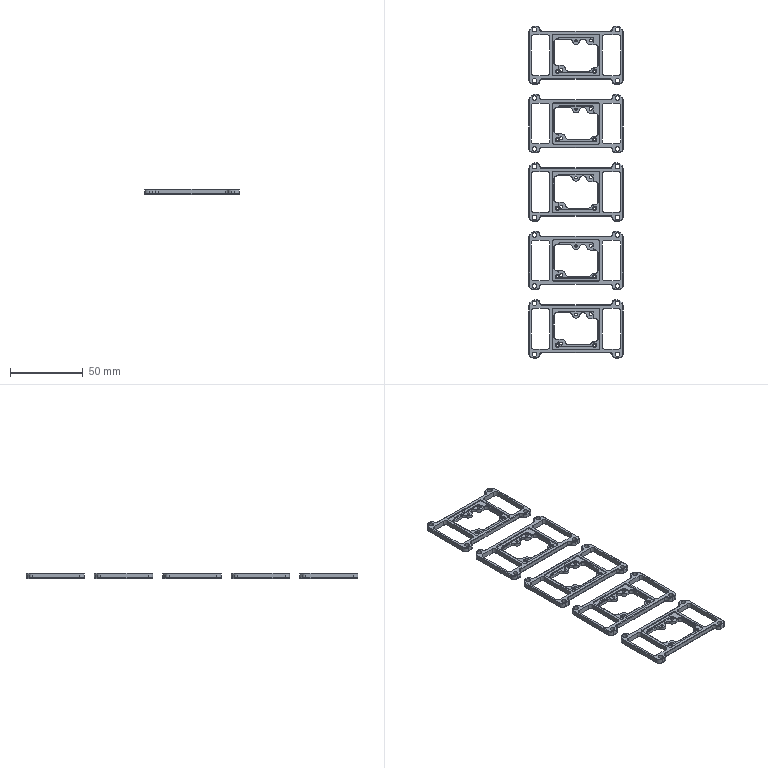NC program | NX | posted with a generic post | part box 65 x 228 x 3.5 mm
Lines 17082 to 18127 of 31259:
(ZLEVEL_PROFILE_COPY_COPY , TOOL : D1.5)
N34126 T17 M6
N34128 G54
N34130 G17 G0 G90 X-80.858 Y13.824 S9500 M3
N34132 G43 Z30. H17
N34134 Z0.4
N34136 G94 G1 Z-0.1 F1000.
N34138 X-80.633 Y13.954
N34140 X-80.552 Y13.994
N34142 X-80.558 Y14.084
N34144 Y15.05
N34146 G3 X-80.95 Y15.442 R0.392
N34148 G1 X-81.916
N34150 X-82.006 Y15.448
N34152 X-82.046 Y15.367
N34154 X-82.176 Y15.142
N34156 Z0.4
N34158 G0 X-80.915 Y13.767 Z0.3
N34160 G1 Z-0.2
N34162 X-80.69 Y13.897
N34164 X-80.61 Y13.936
N34166 X-80.615 Y14.026
N34168 Y15.05
N34170 G3 X-80.95 Y15.385 R0.335
N34172 G1 X-81.974
N34174 X-82.064 Y15.39
N34176 X-82.103 Y15.31
N34178 X-82.233 Y15.085
N34180 Z0.3
N34182 G0 X-80.973 Y13.709 Z0.2
N34184 G1 Z-0.3
N34186 X-80.748 Y13.839
N34188 X-80.667 Y13.879
N34190 X-80.673 Y13.969
N34192 Y15.05
N34194 G3 X-80.95 Y15.327 R0.277
N34196 G1 X-82.031
N34198 X-82.121 Y15.333
N34200 X-82.161 Y15.252
N34202 X-82.291 Y15.027
N34204 Z0.2
N34206 G0 X-81. Y13.682 Z0.1
N34208 G1 Z-0.4
N34210 X-80.775 Y13.812
N34212 X-80.694 Y13.852
N34214 X-80.7 Y13.942
N34216 Y15.05
N34218 G3 X-80.95 Y15.3 R0.25
N34220 G1 X-82.058
N34222 X-82.148 Y15.306
N34224 X-82.188 Y15.225
N34226 X-82.318 Y15.
N34228 Z0.1
N34230 G0 X-81. Y13.682 Z0.
N34232 G1 Z-0.5
N34234 X-80.775 Y13.812
N34236 X-80.694 Y13.852
N34238 X-80.7 Y13.942
N34240 Y15.05
N34242 G3 X-80.95 Y15.3 R0.25
N34244 G1 X-82.058
N34246 X-82.148 Y15.306
N34248 X-82.188 Y15.225
N34250 X-82.318 Y15.
N34252 Z0.
N34254 G0 X-81. Y13.682 Z-0.1
N34256 G1 Z-0.6
N34258 X-80.775 Y13.812
N34260 X-80.694 Y13.852
N34262 X-80.7 Y13.942
N34264 Y15.05
N34266 G3 X-80.95 Y15.3 R0.25
N34268 G1 X-82.058
N34270 X-82.148 Y15.306
N34272 X-82.188 Y15.225
N34274 X-82.318 Y15.
N34276 Z-0.1
N34278 G0 Z10.
N34280 X-105.824 Y15.142
N34282 Z0.4
N34284 G1 Z-0.1
N34286 X-105.954 Y15.367
N34288 X-105.994 Y15.448
N34290 X-106.084 Y15.442
N34292 X-107.05
N34294 G3 X-107.442 Y15.05 R0.392
N34296 G1 Y14.084
N34298 X-107.448 Y13.994
N34300 X-107.367 Y13.954
N34302 X-107.142 Y13.824
N34304 Z0.4
N34306 G0 X-105.767 Y15.085 Z0.3
N34308 G1 Z-0.2
N34310 X-105.897 Y15.31
N34312 X-105.936 Y15.39
N34314 X-106.026 Y15.385
N34316 X-107.05
N34318 G3 X-107.385 Y15.05 R0.335
N34320 G1 Y14.026
N34322 X-107.39 Y13.936
N34324 X-107.31 Y13.897
N34326 X-107.085 Y13.767
N34328 Z0.3
N34330 G0 X-105.709 Y15.027 Z0.2
N34332 G1 Z-0.3
N34334 X-105.839 Y15.252
N34336 X-105.879 Y15.333
N34338 X-105.969 Y15.327
N34340 X-107.05
N34342 G3 X-107.327 Y15.05 R0.277
N34344 G1 Y13.969
N34346 X-107.333 Y13.879
N34348 X-107.252 Y13.839
N34350 X-107.027 Y13.709
N34352 Z0.2
N34354 G0 X-105.682 Y15. Z0.1
N34356 G1 Z-0.4
N34358 X-105.812 Y15.225
N34360 X-105.852 Y15.306
N34362 X-105.942 Y15.3
N34364 X-107.05
N34366 G3 X-107.3 Y15.05 R0.25
N34368 G1 Y13.942
N34370 X-107.306 Y13.852
N34372 X-107.225 Y13.812
N34374 X-107. Y13.682
N34376 Z0.1
N34378 G0 X-105.682 Y15. Z0.
N34380 G1 Z-0.5
N34382 X-105.812 Y15.225
N34384 X-105.852 Y15.306
N34386 X-105.942 Y15.3
N34388 X-107.05
N34390 G3 X-107.3 Y15.05 R0.25
N34392 G1 Y13.942
N34394 X-107.306 Y13.852
N34396 X-107.225 Y13.812
N34398 X-107. Y13.682
N34400 Z0.
N34402 G0 X-105.682 Y15. Z-0.1
N34404 G1 Z-0.6
N34406 X-105.812 Y15.225
N34408 X-105.852 Y15.306
N34410 X-105.942 Y15.3
N34412 X-107.05
N34414 G3 X-107.3 Y15.05 R0.25
N34416 G1 Y13.942
N34418 X-107.306 Y13.852
N34420 X-107.225 Y13.812
N34422 X-107. Y13.682
N34424 Z-0.1
N34426 G0 Z10.
N34428 X-107.142 Y-13.824
N34430 Z0.4
N34432 G1 Z-0.1
N34434 X-107.367 Y-13.954
N34436 X-107.448 Y-13.994
N34438 X-107.442 Y-14.084
N34440 Y-15.05
N34442 G3 X-107.05 Y-15.442 R0.392
N34444 G1 X-106.084
N34446 X-105.994 Y-15.448
N34448 X-105.954 Y-15.367
N34450 X-105.824 Y-15.142
N34452 Z0.4
N34454 G0 X-107.085 Y-13.767 Z0.3
N34456 G1 Z-0.2
N34458 X-107.31 Y-13.897
N34460 X-107.39 Y-13.936
N34462 X-107.385 Y-14.026
N34464 Y-15.05
N34466 G3 X-107.05 Y-15.385 R0.335
N34468 G1 X-106.026
N34470 X-105.936 Y-15.39
N34472 X-105.897 Y-15.31
N34474 X-105.767 Y-15.085
N34476 Z0.3
N34478 G0 X-107.027 Y-13.709 Z0.2
N34480 G1 Z-0.3
N34482 X-107.252 Y-13.839
N34484 X-107.333 Y-13.879
N34486 X-107.327 Y-13.969
N34488 Y-15.05
N34490 G3 X-107.05 Y-15.327 R0.277
N34492 G1 X-105.969
N34494 X-105.879 Y-15.333
N34496 X-105.839 Y-15.252
N34498 X-105.709 Y-15.027
N34500 Z0.2
N34502 G0 X-107. Y-13.682 Z0.1
N34504 G1 Z-0.4
N34506 X-107.225 Y-13.812
N34508 X-107.306 Y-13.852
N34510 X-107.3 Y-13.942
N34512 Y-15.05
N34514 G3 X-107.05 Y-15.3 R0.25
N34516 G1 X-105.942
N34518 X-105.852 Y-15.306
N34520 X-105.812 Y-15.225
N34522 X-105.682 Y-15.
N34524 Z0.1
N34526 G0 X-107. Y-13.682 Z0.
N34528 G1 Z-0.5
N34530 X-107.225 Y-13.812
N34532 X-107.306 Y-13.852
N34534 X-107.3 Y-13.942
N34536 Y-15.05
N34538 G3 X-107.05 Y-15.3 R0.25
N34540 G1 X-105.942
N34542 X-105.852 Y-15.306
N34544 X-105.812 Y-15.225
N34546 X-105.682 Y-15.
N34548 Z0.
N34550 G0 X-107. Y-13.682 Z-0.1
N34552 G1 Z-0.6
N34554 X-107.225 Y-13.812
N34556 X-107.306 Y-13.852
N34558 X-107.3 Y-13.942
N34560 Y-15.05
N34562 G3 X-107.05 Y-15.3 R0.25
N34564 G1 X-105.942
N34566 X-105.852 Y-15.306
N34568 X-105.812 Y-15.225
N34570 X-105.682 Y-15.
N34572 Z-0.1
N34574 G0 Z10.
N34576 X-82.176 Y-15.142
N34578 Z0.4
N34580 G1 Z-0.1
N34582 X-82.046 Y-15.367
N34584 X-82.006 Y-15.448
N34586 X-81.916 Y-15.442
N34588 X-80.95
N34590 G3 X-80.558 Y-15.05 R0.392
N34592 G1 Y-14.084
N34594 X-80.552 Y-13.994
N34596 X-80.633 Y-13.954
N34598 X-80.858 Y-13.824
N34600 Z0.4
N34602 G0 X-82.233 Y-15.085 Z0.3
N34604 G1 Z-0.2
N34606 X-82.103 Y-15.31
N34608 X-82.064 Y-15.39
N34610 X-81.974 Y-15.385
N34612 X-80.95
N34614 G3 X-80.615 Y-15.05 R0.335
N34616 G1 Y-14.026
N34618 X-80.61 Y-13.936
N34620 X-80.69 Y-13.897
N34622 X-80.915 Y-13.767
N34624 Z0.3
N34626 G0 X-82.291 Y-15.027 Z0.2
N34628 G1 Z-0.3
N34630 X-82.161 Y-15.252
N34632 X-82.121 Y-15.333
N34634 X-82.031 Y-15.327
N34636 X-80.95
N34638 G3 X-80.673 Y-15.05 R0.277
N34640 G1 Y-13.969
N34642 X-80.667 Y-13.879
N34644 X-80.748 Y-13.839
N34646 X-80.973 Y-13.709
N34648 Z0.2
N34650 G0 X-82.318 Y-15. Z0.1
N34652 G1 Z-0.4
N34654 X-82.188 Y-15.225
N34656 X-82.148 Y-15.306
N34658 X-82.058 Y-15.3
N34660 X-80.95
N34662 G3 X-80.7 Y-15.05 R0.25
N34664 G1 Y-13.942
N34666 X-80.694 Y-13.852
N34668 X-80.775 Y-13.812
N34670 X-81. Y-13.682
N34672 Z0.1
N34674 G0 X-82.319 Y-15. Z0.
N34676 G1 Z-0.5
N34678 X-82.189 Y-15.225
N34680 X-82.149 Y-15.306
N34682 X-82.059 Y-15.3
N34684 X-80.95
N34686 G3 X-80.7 Y-15.05 R0.25
N34688 G1 Y-13.941
N34690 X-80.694 Y-13.851
N34692 X-80.775 Y-13.811
N34694 X-81. Y-13.681
N34696 Z0.
N34698 G0 X-82.319 Y-15. Z-0.1
N34700 G1 Z-0.6
N34702 X-82.189 Y-15.225
N34704 X-82.149 Y-15.306
N34706 X-82.059 Y-15.3
N34708 X-80.95
N34710 G3 X-80.7 Y-15.05 R0.25
N34712 G1 Y-13.941
N34714 X-80.694 Y-13.851
N34716 X-80.775 Y-13.811
N34718 X-81. Y-13.681
N34720 Z-0.1
N34722 G0 Z10.
N34724 X-76.182 Y28.948
N34726 Z0.4
N34728 G1 Z-0.1
N34730 X-76.37 Y29.275
N34732 X-76.41 Y29.356
N34734 X-76.5 Y29.35
N34736 G3 X-77.35 Y28.5 R0.85
N34738 X-76.5 Y29.35 R-0.85
N34740 G1 X-76.59 Y29.356
N34742 X-76.63 Y29.275
N34744 X-76.818 Y28.948
N34746 Z0.4
N34748 G0 X-76.182 Z0.3
N34750 G1 Z-0.2
N34752 X-76.37 Y29.275
N34754 X-76.41 Y29.356
N34756 X-76.5 Y29.35
N34758 G3 X-77.35 Y28.5 R0.85
N34760 X-76.5 Y29.35 R-0.85
N34762 G1 X-76.59 Y29.356
N34764 X-76.63 Y29.275
N34766 X-76.818 Y28.948
N34768 Z0.3
N34770 G0 X-76.182 Z0.2
N34772 G1 Z-0.3
N34774 X-76.37 Y29.275
N34776 X-76.41 Y29.356
N34778 X-76.5 Y29.35
N34780 G3 X-77.35 Y28.5 R0.85
N34782 X-76.5 Y29.35 R-0.85
N34784 G1 X-76.59 Y29.356
N34786 X-76.63 Y29.275
N34788 X-76.818 Y28.948
N34790 Z0.2
N34792 G0 X-76.182 Z0.1
N34794 G1 Z-0.4
N34796 X-76.37 Y29.275
N34798 X-76.41 Y29.356
N34800 X-76.5 Y29.35
N34802 G3 X-77.35 Y28.5 R0.85
N34804 X-76.5 Y29.35 R-0.85
N34806 G1 X-76.59 Y29.356
N34808 X-76.63 Y29.275
N34810 X-76.818 Y28.948
N34812 Z0.1
N34814 G0 X-76.182 Z0.
N34816 G1 Z-0.5
N34818 X-76.37 Y29.275
N34820 X-76.41 Y29.356
N34822 X-76.5 Y29.35
N34824 G3 X-77.35 Y28.5 R0.85
N34826 X-76.5 Y29.35 R-0.85
N34828 G1 X-76.59 Y29.356
N34830 X-76.63 Y29.275
N34832 X-76.818 Y28.948
N34834 Z0.
N34836 G0 X-76.182 Z-0.1
N34838 G1 Z-0.6
N34840 X-76.37 Y29.275
N34842 X-76.41 Y29.356
N34844 X-76.5 Y29.35
N34846 G3 X-77.35 Y28.5 R0.85
N34848 X-76.5 Y29.35 R-0.85
N34850 G1 X-76.59 Y29.356
N34852 X-76.63 Y29.275
N34854 X-76.818 Y28.948
N34856 Z-0.1
N34858 G0 X-76.182 Z-0.2
N34860 G1 Z-0.7
N34862 X-76.37 Y29.275
N34864 X-76.41 Y29.356
N34866 X-76.5 Y29.35
N34868 G3 X-77.35 Y28.5 R0.85
N34870 X-76.5 Y29.35 R-0.85
N34872 G1 X-76.59 Y29.356
N34874 X-76.63 Y29.275
N34876 X-76.818 Y28.948
N34878 Z-0.2
N34880 G0 X-76.182 Z-0.3
N34882 G1 Z-0.8
N34884 X-76.37 Y29.275
N34886 X-76.41 Y29.356
N34888 X-76.5 Y29.35
N34890 G3 X-77.35 Y28.5 R0.85
N34892 X-76.5 Y29.35 R-0.85
N34894 G1 X-76.59 Y29.356
N34896 X-76.63 Y29.275
N34898 X-76.818 Y28.948
N34900 Z-0.3
N34902 G0 X-76.182 Z-0.4
N34904 G1 Z-0.9
N34906 X-76.37 Y29.275
N34908 X-76.41 Y29.356
N34910 X-76.5 Y29.35
N34912 G3 X-77.35 Y28.5 R0.85
N34914 X-76.5 Y29.35 R-0.85
N34916 G1 X-76.59 Y29.356
N34918 X-76.63 Y29.275
N34920 X-76.818 Y28.948
N34922 Z-0.4
N34924 G0 X-76.182 Z-0.5
N34926 G1 Z-1.
N34928 X-76.37 Y29.275
N34930 X-76.41 Y29.356
N34932 X-76.5 Y29.35
N34934 G3 X-77.35 Y28.5 R0.85
N34936 X-76.5 Y29.35 R-0.85
N34938 G1 X-76.59 Y29.356
N34940 X-76.63 Y29.275
N34942 X-76.818 Y28.948
N34944 Z-0.5
N34946 G0 X-76.182 Z-0.6
N34948 G1 Z-1.1
N34950 X-76.37 Y29.275
N34952 X-76.41 Y29.356
N34954 X-76.5 Y29.35
N34956 G3 X-77.35 Y28.5 R0.85
N34958 X-76.5 Y29.35 R-0.85
N34960 G1 X-76.59 Y29.356
N34962 X-76.63 Y29.275
N34964 X-76.818 Y28.948
N34966 Z-0.6
N34968 G0 X-76.182 Z-0.7
N34970 G1 Z-1.2
N34972 X-76.37 Y29.275
N34974 X-76.41 Y29.356
N34976 X-76.5 Y29.35
N34978 G3 X-77.35 Y28.5 R0.85
N34980 X-76.5 Y29.35 R-0.85
N34982 G1 X-76.59 Y29.356
N34984 X-76.63 Y29.275
N34986 X-76.818 Y28.948
N34988 Z-0.7
N34990 G0 X-76.182 Z-0.8
N34992 G1 Z-1.3
N34994 X-76.37 Y29.275
N34996 X-76.41 Y29.356
N34998 X-76.5 Y29.35
N35000 G3 X-77.35 Y28.5 R0.85
N35002 X-76.5 Y29.35 R-0.85
N35004 G1 X-76.59 Y29.356
N35006 X-76.63 Y29.275
N35008 X-76.818 Y28.948
N35010 Z-0.8
N35012 G0 X-76.182 Z-0.9
N35014 G1 Z-1.4
N35016 X-76.37 Y29.275
N35018 X-76.41 Y29.356
N35020 X-76.5 Y29.35
N35022 G3 X-77.35 Y28.5 R0.85
N35024 X-76.5 Y29.35 R-0.85
N35026 G1 X-76.59 Y29.356
N35028 X-76.63 Y29.275
N35030 X-76.818 Y28.948
N35032 Z-0.9
N35034 G0 X-76.182 Z-1.
N35036 G1 Z-1.5
N35038 X-76.37 Y29.275
N35040 X-76.41 Y29.356
N35042 X-76.5 Y29.35
N35044 G3 X-77.35 Y28.5 R0.85
N35046 X-76.5 Y29.35 R-0.85
N35048 G1 X-76.59 Y29.356
N35050 X-76.63 Y29.275
N35052 X-76.818 Y28.948
N35054 Z-1.
N35056 G0 X-76.182 Z-1.1
N35058 G1 Z-1.6
N35060 X-76.37 Y29.275
N35062 X-76.41 Y29.356
N35064 X-76.5 Y29.35
N35066 G3 X-77.35 Y28.5 R0.85
N35068 X-76.5 Y29.35 R-0.85
N35070 G1 X-76.59 Y29.356
N35072 X-76.63 Y29.275
N35074 X-76.818 Y28.948
N35076 Z-1.1
N35078 G0 X-76.182 Z-1.206
N35080 G1 Z-1.706
N35082 X-76.37 Y29.275
N35084 X-76.41 Y29.356
N35086 X-76.5 Y29.35
N35088 G3 X-77.35 Y28.5 R0.85
N35090 X-76.5 Y29.35 R-0.85
N35092 G1 X-76.59 Y29.356
N35094 X-76.63 Y29.275
N35096 X-76.818 Y28.948
N35098 Z-1.206
N35100 G0 X-76.182 Z-1.311
N35102 G1 Z-1.811
N35104 X-76.37 Y29.275
N35106 X-76.41 Y29.356
N35108 X-76.5 Y29.35
N35110 G3 X-77.35 Y28.5 R0.85
N35112 X-76.5 Y29.35 R-0.85
N35114 G1 X-76.59 Y29.356
N35116 X-76.63 Y29.275
N35118 X-76.818 Y28.948
N35120 Z-1.311
N35122 G0 X-76.182 Z-1.417
N35124 G1 Z-1.917
N35126 X-76.37 Y29.275
N35128 X-76.41 Y29.356
N35130 X-76.5 Y29.35
N35132 G3 X-77.35 Y28.5 R0.85
N35134 X-76.5 Y29.35 R-0.85
N35136 G1 X-76.59 Y29.356
N35138 X-76.63 Y29.275
N35140 X-76.818 Y28.948
N35142 Z-1.417
N35144 G0 X-76.182 Z-1.522
N35146 G1 Z-2.022
N35148 X-76.37 Y29.275
N35150 X-76.41 Y29.356
N35152 X-76.5 Y29.35
N35154 G3 X-77.35 Y28.5 R0.85
N35156 X-76.5 Y29.35 R-0.85
N35158 G1 X-76.59 Y29.356
N35160 X-76.63 Y29.275
N35162 X-76.818 Y28.948
N35164 Z-1.522
N35166 G0 X-76.182 Z-1.628
N35168 G1 Z-2.128
N35170 X-76.37 Y29.275
N35172 X-76.41 Y29.356
N35174 X-76.5 Y29.35
N35176 G3 X-77.35 Y28.5 R0.85
N35178 X-76.5 Y29.35 R-0.85
N35180 G1 X-76.59 Y29.356
N35182 X-76.63 Y29.275
N35184 X-76.818 Y28.948
N35186 Z-1.628
N35188 G0 X-76.182 Z-1.733
N35190 G1 Z-2.233
N35192 X-76.37 Y29.275
N35194 X-76.41 Y29.356
N35196 X-76.5 Y29.35
N35198 G3 X-77.35 Y28.5 R0.85
N35200 X-76.5 Y29.35 R-0.85
N35202 G1 X-76.59 Y29.356
N35204 X-76.63 Y29.275
N35206 X-76.818 Y28.948
N35208 Z-1.733
N35210 G0 X-76.182 Z-1.839
N35212 G1 Z-2.339
N35214 X-76.37 Y29.275
N35216 X-76.41 Y29.356
N35218 X-76.5 Y29.35
N35220 G3 X-77.35 Y28.5 R0.85
N35222 X-76.5 Y29.35 R-0.85
N35224 G1 X-76.59 Y29.356
N35226 X-76.63 Y29.275
N35228 X-76.818 Y28.948
N35230 Z-1.839
N35232 G0 X-76.182 Z-1.944
N35234 G1 Z-2.444
N35236 X-76.37 Y29.275
N35238 X-76.41 Y29.356
N35240 X-76.5 Y29.35
N35242 G3 X-77.35 Y28.5 R0.85
N35244 X-76.5 Y29.35 R-0.85
N35246 G1 X-76.59 Y29.356
N35248 X-76.63 Y29.275
N35250 X-76.818 Y28.948
N35252 Z-1.944
N35254 G0 X-76.182 Z-2.05
N35256 G1 Z-2.55
N35258 X-76.37 Y29.275
N35260 X-76.41 Y29.356
N35262 X-76.5 Y29.35
N35264 G3 X-77.35 Y28.5 R0.85
N35266 X-76.5 Y29.35 R-0.85
N35268 G1 X-76.59 Y29.356
N35270 X-76.63 Y29.275
N35272 X-76.818 Y28.948
N35274 Z-2.05
N35276 G0 X-76.182 Z-2.156
N35278 G1 Z-2.656
N35280 X-76.37 Y29.275
N35282 X-76.41 Y29.356
N35284 X-76.5 Y29.35
N35286 G3 X-77.35 Y28.5 R0.85
N35288 X-76.5 Y29.35 R-0.85
N35290 G1 X-76.59 Y29.356
N35292 X-76.63 Y29.275
N35294 X-76.818 Y28.948
N35296 Z-2.156
N35298 G0 X-76.182 Z-2.261
N35300 G1 Z-2.761
N35302 X-76.37 Y29.275
N35304 X-76.41 Y29.356
N35306 X-76.5 Y29.35
N35308 G3 X-77.35 Y28.5 R0.85
N35310 X-76.5 Y29.35 R-0.85
N35312 G1 X-76.59 Y29.356
N35314 X-76.63 Y29.275
N35316 X-76.818 Y28.948
N35318 Z-2.261
N35320 G0 X-76.182 Z-2.367
N35322 G1 Z-2.867
N35324 X-76.37 Y29.275
N35326 X-76.41 Y29.356
N35328 X-76.5 Y29.35
N35330 G3 X-77.35 Y28.5 R0.85
N35332 X-76.5 Y29.35 R-0.85
N35334 G1 X-76.59 Y29.356
N35336 X-76.63 Y29.275
N35338 X-76.818 Y28.948
N35340 Z-2.367
N35342 G0 X-76.182 Z-2.472
N35344 G1 Z-2.972
N35346 X-76.37 Y29.275
N35348 X-76.41 Y29.356
N35350 X-76.5 Y29.35
N35352 G3 X-77.35 Y28.5 R0.85
N35354 X-76.5 Y29.35 R-0.85
N35356 G1 X-76.59 Y29.356
N35358 X-76.63 Y29.275
N35360 X-76.818 Y28.948
N35362 Z-2.472
N35364 G0 X-76.182 Z-2.578
N35366 G1 Z-3.078
N35368 X-76.37 Y29.275
N35370 X-76.41 Y29.356
N35372 X-76.5 Y29.35
N35374 G3 X-77.35 Y28.5 R0.85
N35376 X-76.5 Y29.35 R-0.85
N35378 G1 X-76.59 Y29.356
N35380 X-76.63 Y29.275
N35382 X-76.818 Y28.948
N35384 Z-2.578
N35386 G0 X-76.182 Z-2.683
N35388 G1 Z-3.183
N35390 X-76.37 Y29.275
N35392 X-76.41 Y29.356
N35394 X-76.5 Y29.35
N35396 G3 X-77.35 Y28.5 R0.85
N35398 X-76.5 Y29.35 R-0.85
N35400 G1 X-76.59 Y29.356
N35402 X-76.63 Y29.275
N35404 X-76.818 Y28.948
N35406 Z-2.683
N35408 G0 X-76.182 Z-2.789
N35410 G1 Z-3.289
N35412 X-76.37 Y29.275
N35414 X-76.41 Y29.356
N35416 X-76.5 Y29.35
N35418 G3 X-77.35 Y28.5 R0.85
N35420 X-76.5 Y29.35 R-0.85
N35422 G1 X-76.59 Y29.356
N35424 X-76.63 Y29.275
N35426 X-76.818 Y28.948
N35428 Z-2.789
N35430 G0 X-76.182 Z-2.894
N35432 G1 Z-3.394
N35434 X-76.37 Y29.275
N35436 X-76.41 Y29.356
N35438 X-76.5 Y29.35
N35440 G3 X-77.35 Y28.5 R0.85
N35442 X-76.5 Y29.35 R-0.85
N35444 G1 X-76.59 Y29.356
N35446 X-76.63 Y29.275
N35448 X-76.818 Y28.948
N35450 Z-2.894
N35452 G0 X-76.182 Z-3.
N35454 G1 Z-3.5
N35456 X-76.37 Y29.275
N35458 X-76.41 Y29.356
N35460 X-76.5 Y29.35
N35462 G3 X-77.35 Y28.5 R0.85
N35464 X-76.5 Y29.35 R-0.85
N35466 G1 X-76.59 Y29.356
N35468 X-76.63 Y29.275
N35470 X-76.818 Y28.948
N35472 Z-3.
N35474 G0 Z10.
N35476 Y-28.948
N35478 Z0.4
N35480 G1 Z-0.1
N35482 X-76.63 Y-29.275
N35484 X-76.59 Y-29.356
N35486 X-76.5 Y-29.35
N35488 X-76.495
N35490 G3 X-75.65 Y-28.495 R0.85
N35492 X-76.5 Y-29.35 R-0.85
N35494 G1 X-76.41 Y-29.356
N35496 X-76.37 Y-29.275
N35498 X-76.182 Y-28.948
N35500 Z0.4
N35502 G0 X-76.818 Z0.3
N35504 G1 Z-0.2
N35506 X-76.63 Y-29.275
N35508 X-76.59 Y-29.356
N35510 X-76.5 Y-29.35
N35512 X-76.495
N35514 G3 X-75.65 Y-28.495 R0.85
N35516 X-76.5 Y-29.35 R-0.85
N35518 G1 X-76.41 Y-29.356
N35520 X-76.37 Y-29.275
N35522 X-76.182 Y-28.948
N35524 Z0.3
N35526 G0 X-76.818 Z0.2
N35528 G1 Z-0.3
N35530 X-76.63 Y-29.275
N35532 X-76.59 Y-29.356
N35534 X-76.5 Y-29.35
N35536 X-76.495
N35538 G3 X-75.65 Y-28.495 R0.85
N35540 X-76.5 Y-29.35 R-0.85
N35542 G1 X-76.41 Y-29.356
N35544 X-76.37 Y-29.275
N35546 X-76.182 Y-28.948
N35548 Z0.2
N35550 G0 X-76.818 Z0.1
N35552 G1 Z-0.4
N35554 X-76.63 Y-29.275
N35556 X-76.59 Y-29.356
N35558 X-76.5 Y-29.35
N35560 X-76.495
N35562 G3 X-75.65 Y-28.495 R0.85
N35564 X-76.5 Y-29.35 R-0.85
N35566 G1 X-76.41 Y-29.356
N35568 X-76.37 Y-29.275
N35570 X-76.182 Y-28.948
N35572 Z0.1
N35574 G0 X-76.818 Z0.
N35576 G1 Z-0.5
N35578 X-76.63 Y-29.275
N35580 X-76.59 Y-29.356
N35582 X-76.5 Y-29.35
N35584 X-76.495
N35586 G3 X-75.65 Y-28.495 R0.85
N35588 X-76.5 Y-29.35 R-0.85
N35590 G1 X-76.41 Y-29.356
N35592 X-76.37 Y-29.275
N35594 X-76.182 Y-28.948
N35596 Z0.
N35598 G0 X-76.818 Z-0.1
N35600 G1 Z-0.6
N35602 X-76.63 Y-29.275
N35604 X-76.59 Y-29.356
N35606 X-76.5 Y-29.35
N35608 X-76.495
N35610 G3 X-75.65 Y-28.495 R0.85
N35612 X-76.5 Y-29.35 R-0.85
N35614 G1 X-76.41 Y-29.356
N35616 X-76.37 Y-29.275
N35618 X-76.182 Y-28.948
N35620 Z-0.1
N35622 G0 X-76.818 Z-0.2
N35624 G1 Z-0.7
N35626 X-76.63 Y-29.275
N35628 X-76.59 Y-29.356
N35630 X-76.5 Y-29.35
N35632 X-76.495
N35634 G3 X-75.65 Y-28.495 R0.85
N35636 X-76.5 Y-29.35 R-0.85
N35638 G1 X-76.41 Y-29.356
N35640 X-76.37 Y-29.275
N35642 X-76.182 Y-28.948
N35644 Z-0.2
N35646 G0 X-76.818 Z-0.3
N35648 G1 Z-0.8
N35650 X-76.63 Y-29.275
N35652 X-76.59 Y-29.356
N35654 X-76.5 Y-29.35
N35656 X-76.495
N35658 G3 X-75.65 Y-28.495 R0.85
N35660 X-76.5 Y-29.35 R-0.85
N35662 G1 X-76.41 Y-29.356
N35664 X-76.37 Y-29.275
N35666 X-76.182 Y-28.948
N35668 Z-0.3
N35670 G0 X-76.818 Z-0.4
N35672 G1 Z-0.9
N35674 X-76.63 Y-29.275
N35676 X-76.59 Y-29.356
N35678 X-76.5 Y-29.35
N35680 X-76.495
N35682 G3 X-75.65 Y-28.495 R0.85
N35684 X-76.5 Y-29.35 R-0.85
N35686 G1 X-76.41 Y-29.356
N35688 X-76.37 Y-29.275
N35690 X-76.182 Y-28.948
N35692 Z-0.4
N35694 G0 X-76.818 Z-0.5
N35696 G1 Z-1.
N35698 X-76.63 Y-29.275
N35700 X-76.59 Y-29.356
N35702 X-76.5 Y-29.35
N35704 X-76.495
N35706 G3 X-75.65 Y-28.495 R0.85
N35708 X-76.5 Y-29.35 R-0.85
N35710 G1 X-76.41 Y-29.356
N35712 X-76.37 Y-29.275
N35714 X-76.182 Y-28.948
N35716 Z-0.5
N35718 G0 X-76.818 Z-0.6
N35720 G1 Z-1.1
N35722 X-76.63 Y-29.275
N35724 X-76.59 Y-29.356
N35726 X-76.5 Y-29.35
N35728 X-76.495
N35730 G3 X-75.65 Y-28.495 R0.85
N35732 X-76.5 Y-29.35 R-0.85
N35734 G1 X-76.41 Y-29.356
N35736 X-76.37 Y-29.275
N35738 X-76.182 Y-28.948
N35740 Z-0.6
N35742 G0 X-76.818 Z-0.7
N35744 G1 Z-1.2
N35746 X-76.63 Y-29.275
N35748 X-76.59 Y-29.356
N35750 X-76.5 Y-29.35
N35752 X-76.495
N35754 G3 X-75.65 Y-28.495 R0.85
N35756 X-76.5 Y-29.35 R-0.85
N35758 G1 X-76.41 Y-29.356
N35760 X-76.37 Y-29.275
N35762 X-76.182 Y-28.948
N35764 Z-0.7
N35766 G0 X-76.818 Z-0.8
N35768 G1 Z-1.3
N35770 X-76.63 Y-29.275
N35772 X-76.59 Y-29.356
N35774 X-76.5 Y-29.35
N35776 X-76.495
N35778 G3 X-75.65 Y-28.495 R0.85
N35780 X-76.5 Y-29.35 R-0.85
N35782 G1 X-76.41 Y-29.356
N35784 X-76.37 Y-29.275
N35786 X-76.182 Y-28.948
N35788 Z-0.8
N35790 G0 X-76.818 Z-0.9
N35792 G1 Z-1.4
N35794 X-76.63 Y-29.275
N35796 X-76.59 Y-29.356
N35798 X-76.5 Y-29.35
N35800 X-76.495
N35802 G3 X-75.65 Y-28.495 R0.85
N35804 X-76.5 Y-29.35 R-0.85
N35806 G1 X-76.41 Y-29.356
N35808 X-76.37 Y-29.275
N35810 X-76.182 Y-28.948
N35812 Z-0.9
N35814 G0 X-76.818 Z-1.
N35816 G1 Z-1.5
N35818 X-76.63 Y-29.275
N35820 X-76.59 Y-29.356
N35822 X-76.5 Y-29.35
N35824 X-76.495
N35826 G3 X-75.65 Y-28.495 R0.85
N35828 X-76.5 Y-29.35 R-0.85
N35830 G1 X-76.41 Y-29.356
N35832 X-76.37 Y-29.275
N35834 X-76.182 Y-28.948
N35836 Z-1.
N35838 G0 X-76.818 Z-1.1
N35840 G1 Z-1.6
N35842 X-76.63 Y-29.275
N35844 X-76.59 Y-29.356
N35846 X-76.5 Y-29.35
N35848 X-76.495
N35850 G3 X-75.65 Y-28.495 R0.85
N35852 X-76.5 Y-29.35 R-0.85
N35854 G1 X-76.41 Y-29.356
N35856 X-76.37 Y-29.275
N35858 X-76.182 Y-28.948
N35860 Z-1.1
N35862 G0 X-76.818 Z-1.206
N35864 G1 Z-1.706
N35866 X-76.63 Y-29.275
N35868 X-76.59 Y-29.356
N35870 X-76.5 Y-29.35
N35872 X-76.495
N35874 G3 X-75.65 Y-28.495 R0.85
N35876 X-76.5 Y-29.35 R-0.85
N35878 G1 X-76.41 Y-29.356
N35880 X-76.37 Y-29.275
N35882 X-76.182 Y-28.948
N35884 Z-1.206
N35886 G0 X-76.818 Z-1.311
N35888 G1 Z-1.811
N35890 X-76.63 Y-29.275
N35892 X-76.59 Y-29.356
N35894 X-76.5 Y-29.35
N35896 X-76.495
N35898 G3 X-75.65 Y-28.495 R0.85
N35900 X-76.5 Y-29.35 R-0.85
N35902 G1 X-76.41 Y-29.356
N35904 X-76.37 Y-29.275
N35906 X-76.182 Y-28.948
N35908 Z-1.311
N35910 G0 X-76.818 Z-1.417
N35912 G1 Z-1.917
N35914 X-76.63 Y-29.275
N35916 X-76.59 Y-29.356
N35918 X-76.5 Y-29.35
N35920 X-76.495
N35922 G3 X-75.65 Y-28.495 R0.85
N35924 X-76.5 Y-29.35 R-0.85
N35926 G1 X-76.41 Y-29.356
N35928 X-76.37 Y-29.275
N35930 X-76.182 Y-28.948
N35932 Z-1.417
N35934 G0 X-76.818 Z-1.522
N35936 G1 Z-2.022
N35938 X-76.63 Y-29.275
N35940 X-76.59 Y-29.356
N35942 X-76.5 Y-29.35
N35944 X-76.495
N35946 G3 X-75.65 Y-28.495 R0.85
N35948 X-76.5 Y-29.35 R-0.85
N35950 G1 X-76.41 Y-29.356
N35952 X-76.37 Y-29.275
N35954 X-76.182 Y-28.948
N35956 Z-1.522
N35958 G0 X-76.818 Z-1.628
N35960 G1 Z-2.128
N35962 X-76.63 Y-29.275
N35964 X-76.59 Y-29.356
N35966 X-76.5 Y-29.35
N35968 X-76.495
N35970 G3 X-75.65 Y-28.495 R0.85
N35972 X-76.5 Y-29.35 R-0.85
N35974 G1 X-76.41 Y-29.356
N35976 X-76.37 Y-29.275
N35978 X-76.182 Y-28.948
N35980 Z-1.628
N35982 G0 X-76.818 Z-1.733
N35984 G1 Z-2.233
N35986 X-76.63 Y-29.275
N35988 X-76.59 Y-29.356
N35990 X-76.5 Y-29.35
N35992 X-76.495
N35994 G3 X-75.65 Y-28.495 R0.85
N35996 X-76.5 Y-29.35 R-0.85
N35998 G1 X-76.41 Y-29.356
N36000 X-76.37 Y-29.275
N36002 X-76.182 Y-28.948
N36004 Z-1.733
N36006 G0 X-76.818 Z-1.839
N36008 G1 Z-2.339
N36010 X-76.63 Y-29.275
N36012 X-76.59 Y-29.356
N36014 X-76.5 Y-29.35
N36016 X-76.495
N36018 G3 X-75.65 Y-28.495 R0.85
N36020 X-76.5 Y-29.35 R-0.85
N36022 G1 X-76.41 Y-29.356
N36024 X-76.37 Y-29.275
N36026 X-76.182 Y-28.948
N36028 Z-1.839
N36030 G0 X-76.818 Z-1.944
N36032 G1 Z-2.444
N36034 X-76.63 Y-29.275
N36036 X-76.59 Y-29.356
N36038 X-76.5 Y-29.35
N36040 X-76.495
N36042 G3 X-75.65 Y-28.495 R0.85
N36044 X-76.5 Y-29.35 R-0.85
N36046 G1 X-76.41 Y-29.356
N36048 X-76.37 Y-29.275
N36050 X-76.182 Y-28.948
N36052 Z-1.944
N36054 G0 X-76.818 Z-2.05
N36056 G1 Z-2.55
N36058 X-76.63 Y-29.275
N36060 X-76.59 Y-29.356
N36062 X-76.5 Y-29.35
N36064 X-76.495
N36066 G3 X-75.65 Y-28.495 R0.85
N36068 X-76.5 Y-29.35 R-0.85
N36070 G1 X-76.41 Y-29.356
N36072 X-76.37 Y-29.275
N36074 X-76.182 Y-28.948
N36076 Z-2.05
N36078 G0 X-76.818 Z-2.156
N36080 G1 Z-2.656
N36082 X-76.63 Y-29.275
N36084 X-76.59 Y-29.356
N36086 X-76.5 Y-29.35
N36088 X-76.495
N36090 G3 X-75.65 Y-28.495 R0.85
N36092 X-76.5 Y-29.35 R-0.85
N36094 G1 X-76.41 Y-29.356
N36096 X-76.37 Y-29.275
N36098 X-76.182 Y-28.948
N36100 Z-2.156
N36102 G0 X-76.818 Z-2.261
N36104 G1 Z-2.761
N36106 X-76.63 Y-29.275
N36108 X-76.59 Y-29.356
N36110 X-76.5 Y-29.35
N36112 X-76.495
N36114 G3 X-75.65 Y-28.495 R0.85
N36116 X-76.5 Y-29.35 R-0.85
N36118 G1 X-76.41 Y-29.356
N36120 X-76.37 Y-29.275
N36122 X-76.182 Y-28.948
N36124 Z-2.261
N36126 G0 X-76.818 Z-2.367
N36128 G1 Z-2.867
N36130 X-76.63 Y-29.275
N36132 X-76.59 Y-29.356
N36134 X-76.5 Y-29.35
N36136 X-76.495
N36138 G3 X-75.65 Y-28.495 R0.85
N36140 X-76.5 Y-29.35 R-0.85
N36142 G1 X-76.41 Y-29.356
N36144 X-76.37 Y-29.275
N36146 X-76.182 Y-28.948
N36148 Z-2.367
N36150 G0 X-76.818 Z-2.472
N36152 G1 Z-2.972
N36154 X-76.63 Y-29.275
N36156 X-76.59 Y-29.356
N36158 X-76.5 Y-29.35
N36160 X-76.495
N36162 G3 X-75.65 Y-28.495 R0.85
N36164 X-76.5 Y-29.35 R-0.85
N36166 G1 X-76.41 Y-29.356
N36168 X-76.37 Y-29.275
N36170 X-76.182 Y-28.948
N36172 Z-2.472
N36174 G0 X-76.818 Z-2.578
N36176 G1 Z-3.078
N36178 X-76.63 Y-29.275
N36180 X-76.59 Y-29.356
N36182 X-76.5 Y-29.35
N36184 X-76.495
N36186 G3 X-75.65 Y-28.495 R0.85
N36188 X-76.5 Y-29.35 R-0.85
N36190 G1 X-76.41 Y-29.356
N36192 X-76.37 Y-29.275
N36194 X-76.182 Y-28.948
N36196 Z-2.578
N36198 G0 X-76.818 Z-2.683
N36200 G1 Z-3.183
N36202 X-76.63 Y-29.275
N36204 X-76.59 Y-29.356
N36206 X-76.5 Y-29.35
N36208 X-76.495
N36210 G3 X-75.65 Y-28.495 R0.85